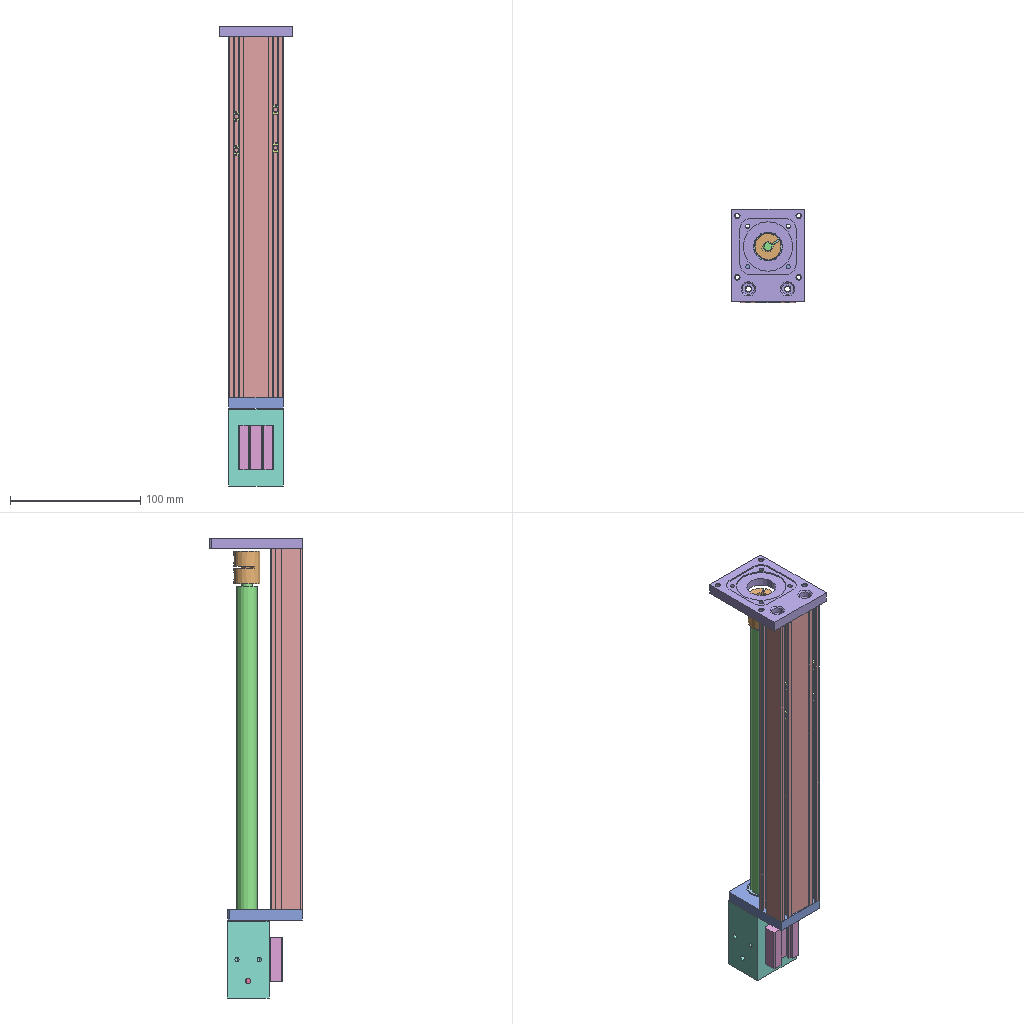Assembly | SolidWorks | 11 different items | 14 placed | box 56 x 71 x 353 mm
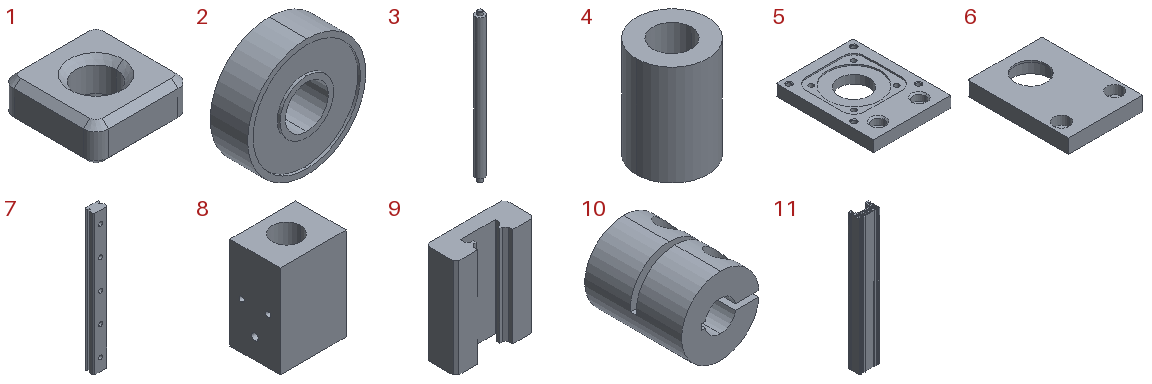Parts list (item | quantity | size | volume | features):
1 | x4 | 7.6 x 7.6 x 3 mm | 135.283 mm3 | features Chamfer 3, Extrusion 1, HoleWzd 1
2 | x1 | 22 x 7 x 22 mm | 2073 mm3 | features ICE 2, Extrusion 1
3 | x1 | 16 x 16 x 264 mm | 50645 mm3 | features ICE 2, Chamfer 1, Extrusion 1, Helix 1
4 | x1 | 27 x 27 x 38 mm | 15482 mm3 | features Extrusion 1, HoleWzd 1
5 | x1 | 56 x 71 x 8 mm | 24816 mm3 | features Chamfer 5, ICE 4, Extrusion 1, HoleWzd 1
6 | x1 | 42 x 57 x 8 mm | 15479 mm3 | features ICE 2, Extrusion 1
7 | x1 | 12 x 8 x 121 mm | 9982 mm3 | features ICE 2, Extrusion 1
8 | x1 | 42 x 32 x 59 mm | 49987 mm3 | features HoleWzd 3, ICE 2, Extrusion 1, MirrorPattern 1
9 | x1 | 27 x 10.5 x 34 mm | 7327 mm3 | features Chamfer 1, Extrusion 1
10 | x1 | 19.972 x 25 x 20 mm | 5780 mm3 | features ICE 4, Extrusion 1, HoleWzd 1
11 | x1 | 42 x 24.4 x 277 mm | 94986 mm3 | features Extrusion 1, WeldmentFeature 1
Mates (type | each side: item.copy, entity, surface, feature):
Concentric | 6.1 face cylinder Cut-Extrude2 | 2.1 face cylinder Boss-Extrude1
Coincident | 6.1 edge | 2.1 edge
Coincident | 11.1 face plane Boss-Extrude1 | 6.1 face plane Boss-Extrude1
Coincident | 11.1 edge | 6.1 edge | 2 times
Concentric | 8.1 face cylinder Cut-Extrude1 | 4.1 face cylinder Boss-Extrude1
Coincident | 8.1 edge | 4.1 edge
Coincident | 11.1 face plane Boss-Extrude1 | 5.1 face plane Boss-Extrude1
Coincident | 11.1 edge | 5.1 edge
Concentric | 11.1 edge | 5.1 edge
Coincident | 11.1 face plane Boss-Extrude1 | 7.1 face plane Boss-Extrude1
Coincident | 6.1 face plane Boss-Extrude1 | 7.1 face plane Boss-Extrude1
Concentric | 3.1 face cylinder Boss-Extrude3 | 2.1 face cylinder Boss-Extrude1
Coincident | 3.1 edge | 2.1 edge
Concentric | 10.1 face cylinder Boss-Extrude1 | 3.1 face cylinder Boss-Extrude2
Coincident | 7.1 face plane Boss-Extrude1 | 9.1 face plane Boss-Extrude1
DistanceDim | 7.1 face plane Boss-Extrude1 | 9.1 face plane Boss-Extrude1
DistanceDim | 9.1 edge | 8.1 edge | 2 times
Concentric | 8.1 edge | 5.1 edge
Coincident | 11.1 face plane Boss-Extrude1 | 1.1 face plane Boss-Extrude1
DistanceDim | 1.1 face plane Boss-Extrude1 | 11.1 face plane Boss-Extrude1
Coincident | 11.1 face plane Boss-Extrude1 | 1.2 face plane Boss-Extrude1
DistanceDim | 1.2 face plane Boss-Extrude1 | 11.1 face plane Boss-Extrude1
Coincident | 11.1 face plane Boss-Extrude1 | 1.3 face plane Boss-Extrude1
Coincident | 11.1 face plane Boss-Extrude1 | 1.4 face plane Boss-Extrude1
DistanceDim | 11.1 face plane Boss-Extrude1 | 1.4 face plane Boss-Extrude1
DistanceDim | 11.1 face plane Boss-Extrude1 | 1.3 face plane Boss-Extrude1